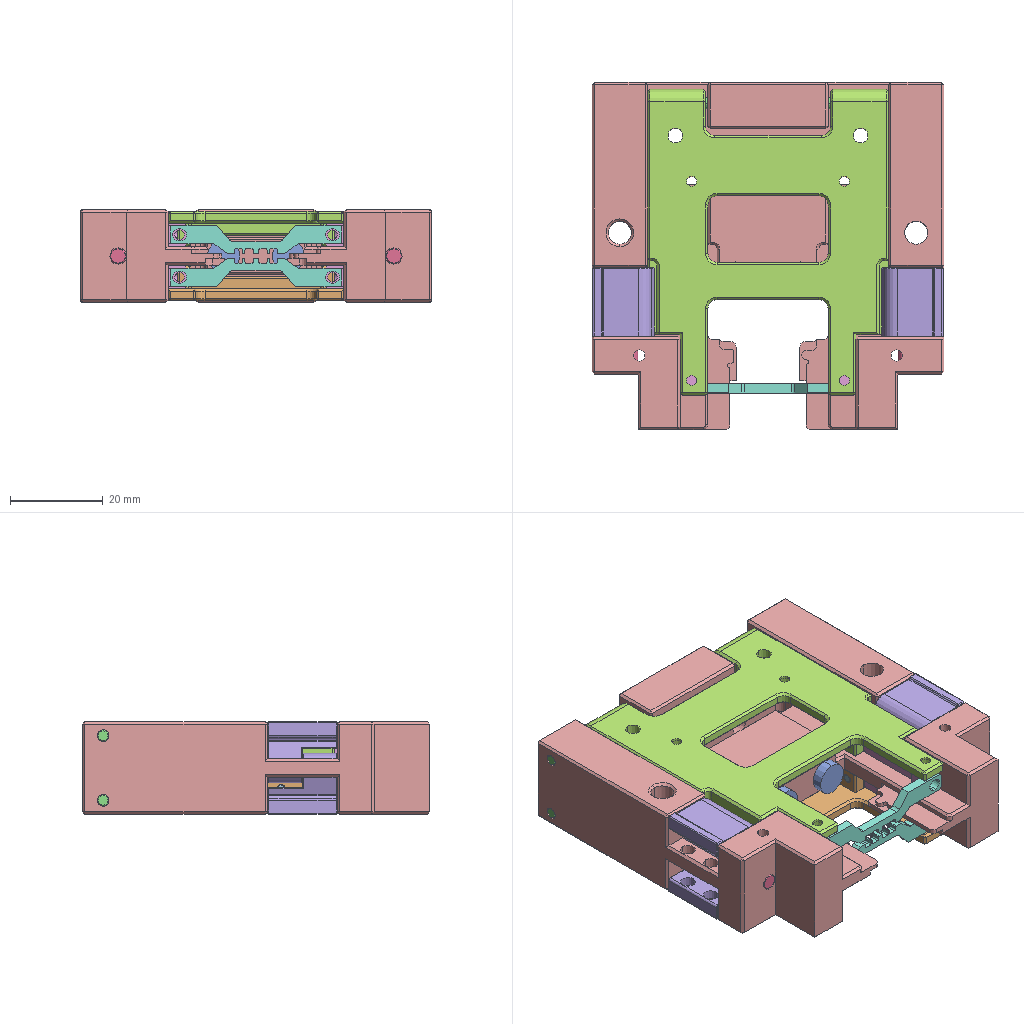Assembly | SolidWorks | 12 different items | 25 placed | box 76 x 75 x 20 mm
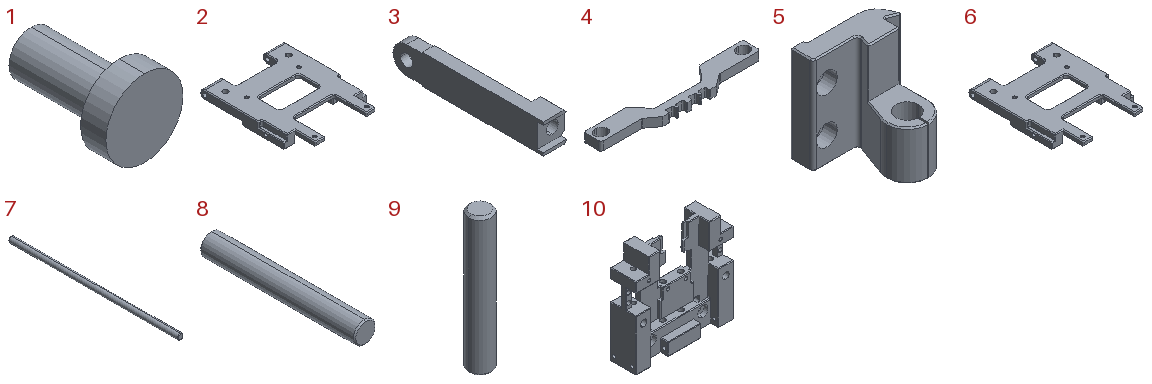Parts list (item | name | quantity | size | volume | features):
1 | - | x2 | 7 x 10.3 x 7 mm | 189.045 mm3 | features Extrusion 1, ICE 1
2 | - | x1 | 52 x 66.1 x 7.6 mm | 7864 mm3 | features ICE 16, Fillet 6, Chamfer 2, MoveFace 2, Cut 1, DelFace 1, Extrusion 1
3 | - | x4 | 4.5 x 25.5 x 5 mm | 257.777 mm3 | features ICE 4, Chamfer 1, Extrusion 1, Fillet 1, HoleWzd 1
4 | - | x2 | 37 x 6.09 x 2 mm | 221.807 mm3 | features ICE 5, Fillet 2, Chamfer 1, Extrusion 1
5 | - | x4 | 13.215 x 13.198 x 14.95 mm | 916.402 mm3 | features Fillet 6, ICE 5, Chamfer 1, Extrusion 1
6 | - | x1 | 52 x 66.1 x 7.6 mm | 7860 mm3 | features ICE 17, Fillet 6, Chamfer 2, MoveFace 2, Extrusion 1
7 | - | x2 | 2.5 x 76 x 2.5 mm | 372.767 mm3 | features Chamfer 1, Extrusion 1
8 | - | x2 | 3.5 x 25 x 3.5 mm | 240.105 mm3 | features Chamfer 1, Extrusion 1
9 | - | x4 | 2 x 2 x 12 mm | 37.465 mm3 | features Chamfer 1, Extrusion 1
10 | - | x1 | 76 x 20 x 75 mm | 45299 mm3 | features ICE 34, Fillet 3, HoleWzd 3, Chamfer 2, Cut 2, Extrusion 1
11 | PCB | x1 | - | - | -
12 | Dust Cap | x1 | - | - | -
Mates (type | each side: item.copy, entity, surface, feature):
Concentric | 10.1 face cylinder Cut-Extrude15 | 1.1 face cylinder Boss-Extrude1
Coincident | 10.1 face plane Boss-Extrude6 | 1.1 face plane Boss-Extrude2
Concentric | 10.1 face cylinder Cut-Extrude16 | 2.1 face cylinder Cut-Extrude2
Coincident | 10.1 face plane Cut-Extrude6 | 2.1 face plane Boss-Extrude1
LimitPlanarAngleDim | 2.1 face plane Boss-Extrude1 | 10.1 face plane Cut-Extrude2
Concentric | 10.1 face cylinder Cut-Extrude33 | 5.1 face cylinder Boss-Extrude1
Coincident | 10.1 face plane Cut-Extrude2 | 5.1 face plane Boss-Extrude1
Concentric | 10.1 face cylinder Cut-Extrude33 | 5.2 face cylinder Boss-Extrude1
Coincident | 10.1 face plane Cut-Extrude2 | 5.2 face plane Boss-Extrude1
Concentric | 10.1 face cylinder Cut-Extrude33 | 5.3 face cylinder Boss-Extrude1
Coincident | 10.1 face plane Cut-Extrude2 | 5.3 face plane Boss-Extrude1
Concentric | 10.1 face cylinder Cut-Extrude33 | 5.4 face cylinder Boss-Extrude1
Coincident | 10.1 face plane Cut-Extrude2 | 5.4 face plane Boss-Extrude1
Parallel | 10.1 face plane Boss-Extrude1 | 5.4 face plane Boss-Extrude1
Parallel | 10.1 face plane Boss-Extrude1 | 5.3 face plane Boss-Extrude1
Parallel | 10.1 face plane Boss-Extrude1 | 5.1 face plane Boss-Extrude1
Parallel | 10.1 face plane Boss-Extrude1 | 5.2 face plane Boss-Extrude1
Concentric | 10.1 face cylinder Cut-Extrude16 | 7.1 face cylinder Boss-Extrude1
Concentric | 10.1 face cylinder Cut-Extrude16 | 7.2 face cylinder Boss-Extrude1
Coincident | 10.1 face plane Boss-Extrude1 | 7.1 face plane Boss-Extrude1
Coincident | 10.1 face plane Boss-Extrude1 | 7.2 face plane Boss-Extrude1
Concentric | 10.1 face cylinder Cut-Extrude33 | 8.1 face cylinder Boss-Extrude1
Coincident | 10.1 face plane Cut-Extrude1 | 8.1 edge
Concentric | 10.1 face cylinder Cut-Extrude33 | 8.2 face cylinder Boss-Extrude1
Coincident | 10.1 face plane Cut-Extrude1 | 8.2 face plane Boss-Extrude1
Concentric | 10.1 face cylinder Cut-Extrude15 | 1.2 face cylinder Boss-Extrude1
Coincident | 10.1 face plane Boss-Extrude6 | 1.2 face plane Boss-Extrude2
Coincident | 3.1 face plane Cut-Extrude1 | 2.1 face plane Cut-Extrude1
Coincident | 3.2 face plane Cut-Extrude1 | 2.1 face plane Cut-Extrude1
Coincident | 3.2 face plane Cut-Extrude4 | 4.1 face plane Boss-Extrude1 | 2 times
LimitPlanarAngleDim | 3.2 face plane Boss-Extrude1 | 2.1 face plane Cut-Extrude1
Parallel | 3.1 face plane Boss-Extrude1 | 3.2 face plane Boss-Extrude1
DistanceDim | 3.2 face plane Boss-Extrude1 | 4.1 face plane Boss-Extrude1
Concentric | 3.3 face cylinder Cut-Extrude2 | 9.1 face cylinder Boss-Extrude1
Concentric | 9.2 face cylinder Boss-Extrude1 | 3.4 face cylinder Cut-Extrude2
Parallel | 3.3 face plane Boss-Extrude1 | 3.4 face plane Boss-Extrude1
Coincident | 4.2 face plane Boss-Extrude1 | 3.4 face plane Cut-Extrude4 | 2 times
DistanceDim | 4.2 face plane Boss-Extrude1 | 3.3 face plane Boss-Extrude1
Coincident | 10.1 face plane Cut-Extrude13 | 6.1 face plane Boss-Extrude1
Concentric | 6.1 face cylinder Cut-Extrude2 | 7.1 face cylinder Boss-Extrude1
Concentric | 6.1 face cylinder Cut-Extrude4 | 9.1 face cylinder Boss-Extrude1
Concentric | 6.1 face cylinder Cut-Extrude4 | 9.2 face cylinder Boss-Extrude1
LimitPlanarAngleDim | 6.1 face plane Cut-Extrude5 | 10.1 face plane Cut-Extrude13
Coincident | 6.1 face plane Cut-Extrude1 | 3.3 face plane Boss-Extrude1
LimitPlanarAngleDim | 3.4 face plane Boss-Extrude1 | 6.1 face plane Cut-Extrude1
Coincident | 6.1 face plane Cut-Extrude1 | 3.4 face plane Boss-Extrude1
Coincident | 6.1 face plane Cut-Extrude21 | 9.2 face plane Boss-Extrude1
Coincident | 6.1 face plane Cut-Extrude21 | 9.1 edge
Concentric | 2.1 face cylinder Cut-Extrude4 | 9.3 face cylinder Boss-Extrude1
Coincident | 2.1 face plane Cut-Extrude21 | 9.3 face plane Boss-Extrude1
Concentric | 2.1 face cylinder Cut-Extrude4 | 9.4 face cylinder Boss-Extrude1
Coincident | 2.1 face plane Cut-Extrude21 | 9.4 face plane Boss-Extrude1
Concentric | 2.1 face cylinder Cut-Extrude4 | 3.2 face cylinder Cut-Extrude2
Concentric | 3.1 face cylinder Cut-Extrude2 | 2.1 face cylinder Cut-Extrude4